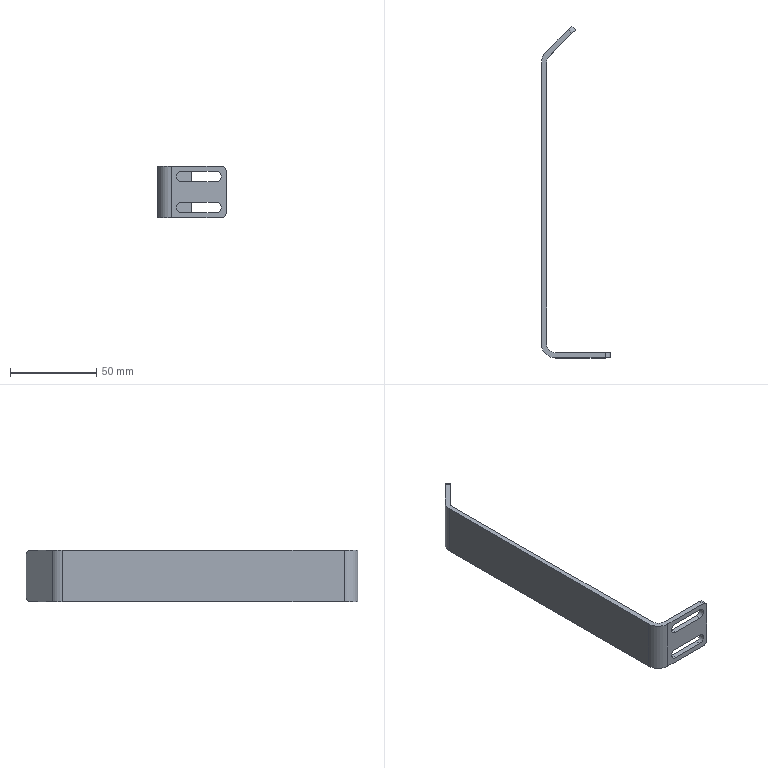Part | NX | features BREP 1 | 1 solid | 26 faces | box 40 x 192.678 x 30 mm | volume 20029 mm3 | plane 14 | cylinder 12 | commonest cylinder face diameters 6 x8 10 x2 16 x2
STEP:
#1=CARTESIAN_POINT('',(0.,8.,30.));
#2=VERTEX_POINT('',#1);
#3=CARTESIAN_POINT('',(0.,171.686,30.));
#4=VERTEX_POINT('',#3);
#5=CARTESIAN_POINT('',(0.,0.,30.));
#6=DIRECTION('',(0.,1.,0.));
#7=VECTOR('',#6,1000.);
#8=LINE('',#5,#7);
#9=EDGE_CURVE('',#2,#4,#8,.T.);
#10=ORIENTED_EDGE('',*,*,#9,.T.);
#11=CARTESIAN_POINT('',(0.,171.686,0.));
#12=VERTEX_POINT('',#11);
#13=CARTESIAN_POINT('',(0.,171.686,30.));
#14=DIRECTION('',(0.,0.,-1.));
#15=VECTOR('',#14,1000.);
#16=LINE('',#13,#15);
#17=EDGE_CURVE('',#4,#12,#16,.T.);
#18=ORIENTED_EDGE('',*,*,#17,.T.);
#19=CARTESIAN_POINT('',(0.,8.,0.));
#20=VERTEX_POINT('',#19);
#21=CARTESIAN_POINT('',(0.,0.,0.));
#22=DIRECTION('',(0.,-1.,0.));
#23=VECTOR('',#22,1000.);
#24=LINE('',#21,#23);
#25=EDGE_CURVE('',#12,#20,#24,.T.);
#26=ORIENTED_EDGE('',*,*,#25,.T.);
#27=CARTESIAN_POINT('',(0.,8.,30.));
#28=DIRECTION('',(0.,0.,1.));
#29=VECTOR('',#28,1000.);
#30=LINE('',#27,#29);
#31=EDGE_CURVE('',#20,#2,#30,.T.);
#32=ORIENTED_EDGE('',*,*,#31,.T.);
#33=EDGE_LOOP('',(#10,#18,#26,#32));
#34=FACE_BOUND('',#33,.T.);
#35=CARTESIAN_POINT('',(0.,0.,30.));
#36=DIRECTION('',(-1.,0.,0.));
#37=DIRECTION('',(0.,0.,-1.));
#38=AXIS2_PLACEMENT_3D('',#35,#36,#37);
#39=PLANE('',#38);
#40=ADVANCED_FACE('',(#34),#39,.T.);
#41=CARTESIAN_POINT('',(2.343,177.343,30.));
#42=VERTEX_POINT('',#41);
#43=CARTESIAN_POINT('',(8.,171.686,30.));
#44=DIRECTION('',(0.,0.,-1.));
#45=DIRECTION('',(-1.,0.,0.));
#46=AXIS2_PLACEMENT_3D('',#43,#44,#45);
#47=CIRCLE('',#46,8.);
#48=EDGE_CURVE('',#4,#42,#47,.T.);
#49=ORIENTED_EDGE('',*,*,#48,.T.);
#50=CARTESIAN_POINT('',(2.343,177.343,0.));
#51=VERTEX_POINT('',#50);
#52=CARTESIAN_POINT('',(2.343,177.343,30.));
#53=DIRECTION('',(0.,0.,-1.));
#54=VECTOR('',#53,1000.);
#55=LINE('',#52,#54);
#56=EDGE_CURVE('',#42,#51,#55,.T.);
#57=ORIENTED_EDGE('',*,*,#56,.T.);
#58=CARTESIAN_POINT('',(8.,171.686,0.));
#59=DIRECTION('',(0.,0.,1.));
#60=DIRECTION('',(-1.,0.,0.));
#61=AXIS2_PLACEMENT_3D('',#58,#59,#60);
#62=CIRCLE('',#61,8.);
#63=EDGE_CURVE('',#51,#12,#62,.T.);
#64=ORIENTED_EDGE('',*,*,#63,.T.);
#65=ORIENTED_EDGE('',*,*,#17,.F.);
#66=EDGE_LOOP('',(#49,#57,#64,#65));
#67=FACE_BOUND('',#66,.T.);
#68=CARTESIAN_POINT('',(8.,171.686,30.));
#69=DIRECTION('',(0.,0.,-1.));
#70=DIRECTION('',(1.,0.,0.));
#71=AXIS2_PLACEMENT_3D('',#68,#69,#70);
#72=CYLINDRICAL_SURFACE('',#71,8.);
#73=ADVANCED_FACE('',(#67),#72,.T.);
#74=CARTESIAN_POINT('',(3.,8.,30.));
#75=VERTEX_POINT('',#74);
#76=CARTESIAN_POINT('',(3.,171.686,30.));
#77=VERTEX_POINT('',#76);
#78=CARTESIAN_POINT('',(3.,3.,30.));
#79=DIRECTION('',(0.,1.,0.));
#80=VECTOR('',#79,1000.);
#81=LINE('',#78,#80);
#82=EDGE_CURVE('',#75,#77,#81,.T.);
#83=ORIENTED_EDGE('',*,*,#82,.T.);
#84=CARTESIAN_POINT('',(4.464,175.222,30.));
#85=VERTEX_POINT('',#84);
#86=CARTESIAN_POINT('',(8.,171.686,30.));
#87=DIRECTION('',(0.,0.,-1.));
#88=DIRECTION('',(-1.,0.,0.));
#89=AXIS2_PLACEMENT_3D('',#86,#87,#88);
#90=CIRCLE('',#89,5.);
#91=EDGE_CURVE('',#77,#85,#90,.T.);
#92=ORIENTED_EDGE('',*,*,#91,.T.);
#93=CARTESIAN_POINT('',(17.678,188.435,30.));
#94=VERTEX_POINT('',#93);
#95=CARTESIAN_POINT('',(4.464,175.222,30.));
#96=DIRECTION('',(0.7071,0.7071,0.));
#97=VECTOR('',#96,1000.);
#98=LINE('',#95,#97);
#99=EDGE_CURVE('',#85,#94,#98,.T.);
#100=ORIENTED_EDGE('',*,*,#99,.T.);
#101=CARTESIAN_POINT('',(15.556,190.556,30.));
#102=VERTEX_POINT('',#101);
#103=CARTESIAN_POINT('',(15.556,190.556,30.));
#104=DIRECTION('',(0.7071,-0.7071,0.));
#105=VECTOR('',#104,1000.);
#106=LINE('',#103,#105);
#107=EDGE_CURVE('',#102,#94,#106,.T.);
#108=ORIENTED_EDGE('',*,*,#107,.F.);
#109=CARTESIAN_POINT('',(0.,175.,30.));
#110=DIRECTION('',(0.7071,0.7071,0.));
#111=VECTOR('',#110,1000.);
#112=LINE('',#109,#111);
#113=EDGE_CURVE('',#42,#102,#112,.T.);
#114=ORIENTED_EDGE('',*,*,#113,.F.);
#115=ORIENTED_EDGE('',*,*,#48,.F.);
#116=ORIENTED_EDGE('',*,*,#9,.F.);
#117=CARTESIAN_POINT('',(8.,0.,30.));
#118=VERTEX_POINT('',#117);
#119=CARTESIAN_POINT('',(8.,8.,30.));
#120=DIRECTION('',(0.,0.,-1.));
#121=DIRECTION('',(-1.,0.,0.));
#122=AXIS2_PLACEMENT_3D('',#119,#120,#121);
#123=CIRCLE('',#122,8.);
#124=EDGE_CURVE('',#118,#2,#123,.T.);
#125=ORIENTED_EDGE('',*,*,#124,.F.);
#126=CARTESIAN_POINT('',(37.,0.,30.));
#127=VERTEX_POINT('',#126);
#128=CARTESIAN_POINT('',(40.,0.,30.));
#129=DIRECTION('',(-1.,0.,0.));
#130=VECTOR('',#129,1000.);
#131=LINE('',#128,#130);
#132=EDGE_CURVE('',#127,#118,#131,.T.);
#133=ORIENTED_EDGE('',*,*,#132,.F.);
#134=CARTESIAN_POINT('',(37.,3.,30.));
#135=VERTEX_POINT('',#134);
#136=CARTESIAN_POINT('',(37.,171.686,30.));
#137=DIRECTION('',(0.,1.,0.));
#138=VECTOR('',#137,1000.);
#139=LINE('',#136,#138);
#140=EDGE_CURVE('',#127,#135,#139,.T.);
#141=ORIENTED_EDGE('',*,*,#140,.T.);
#142=CARTESIAN_POINT('',(8.,3.,30.));
#143=VERTEX_POINT('',#142);
#144=CARTESIAN_POINT('',(8.,3.,30.));
#145=DIRECTION('',(-1.,0.,0.));
#146=VECTOR('',#145,1000.);
#147=LINE('',#144,#146);
#148=EDGE_CURVE('',#135,#143,#147,.T.);
#149=ORIENTED_EDGE('',*,*,#148,.T.);
#150=CARTESIAN_POINT('',(8.,8.,30.));
#151=DIRECTION('',(0.,0.,-1.));
#152=DIRECTION('',(-1.,0.,0.));
#153=AXIS2_PLACEMENT_3D('',#150,#151,#152);
#154=CIRCLE('',#153,5.);
#155=EDGE_CURVE('',#143,#75,#154,.T.);
#156=ORIENTED_EDGE('',*,*,#155,.T.);
#157=EDGE_LOOP('',(#83,#92,#100,#108,#114,#115,#116,#125,#133,#141,#149,#156));
#158=FACE_BOUND('',#157,.T.);
#159=CARTESIAN_POINT('',(8.,3.,30.));
#160=DIRECTION('',(0.,0.,1.));
#161=DIRECTION('',(-1.,0.,0.));
#162=AXIS2_PLACEMENT_3D('',#159,#160,#161);
#163=PLANE('',#162);
#164=ADVANCED_FACE('',(#158),#163,.T.);
#165=ORIENTED_EDGE('',*,*,#124,.T.);
#166=ORIENTED_EDGE('',*,*,#31,.F.);
#167=CARTESIAN_POINT('',(8.,0.,0.));
#168=VERTEX_POINT('',#167);
#169=CARTESIAN_POINT('',(8.,8.,0.));
#170=DIRECTION('',(0.,0.,1.));
#171=DIRECTION('',(-1.,0.,0.));
#172=AXIS2_PLACEMENT_3D('',#169,#170,#171);
#173=CIRCLE('',#172,8.);
#174=EDGE_CURVE('',#20,#168,#173,.T.);
#175=ORIENTED_EDGE('',*,*,#174,.T.);
#176=CARTESIAN_POINT('',(8.,0.,30.));
#177=DIRECTION('',(0.,0.,1.));
#178=VECTOR('',#177,1000.);
#179=LINE('',#176,#178);
#180=EDGE_CURVE('',#168,#118,#179,.T.);
#181=ORIENTED_EDGE('',*,*,#180,.T.);
#182=EDGE_LOOP('',(#165,#166,#175,#181));
#183=FACE_BOUND('',#182,.T.);
#184=CARTESIAN_POINT('',(8.,8.,30.));
#185=DIRECTION('',(0.,0.,-1.));
#186=DIRECTION('',(1.,0.,0.));
#187=AXIS2_PLACEMENT_3D('',#184,#185,#186);
#188=CYLINDRICAL_SURFACE('',#187,8.);
#189=ADVANCED_FACE('',(#183),#188,.T.);
#190=CARTESIAN_POINT('',(3.,171.686,0.));
#191=VERTEX_POINT('',#190);
#192=CARTESIAN_POINT('',(3.,8.,0.));
#193=VERTEX_POINT('',#192);
#194=CARTESIAN_POINT('',(3.,175.222,0.));
#195=DIRECTION('',(0.,-1.,0.));
#196=VECTOR('',#195,1000.);
#197=LINE('',#194,#196);
#198=EDGE_CURVE('',#191,#193,#197,.T.);
#199=ORIENTED_EDGE('',*,*,#198,.T.);
#200=CARTESIAN_POINT('',(8.,3.,0.));
#201=VERTEX_POINT('',#200);
#202=CARTESIAN_POINT('',(8.,8.,0.));
#203=DIRECTION('',(0.,0.,1.));
#204=DIRECTION('',(-1.,0.,0.));
#205=AXIS2_PLACEMENT_3D('',#202,#203,#204);
#206=CIRCLE('',#205,5.);
#207=EDGE_CURVE('',#193,#201,#206,.T.);
#208=ORIENTED_EDGE('',*,*,#207,.T.);
#209=CARTESIAN_POINT('',(37.,3.,0.));
#210=VERTEX_POINT('',#209);
#211=CARTESIAN_POINT('',(3.,3.,0.));
#212=DIRECTION('',(1.,0.,0.));
#213=VECTOR('',#212,1000.);
#214=LINE('',#211,#213);
#215=EDGE_CURVE('',#201,#210,#214,.T.);
#216=ORIENTED_EDGE('',*,*,#215,.T.);
#217=CARTESIAN_POINT('',(37.,0.,0.));
#218=VERTEX_POINT('',#217);
#219=CARTESIAN_POINT('',(37.,8.,0.));
#220=DIRECTION('',(0.,1.,0.));
#221=VECTOR('',#220,1000.);
#222=LINE('',#219,#221);
#223=EDGE_CURVE('',#218,#210,#222,.T.);
#224=ORIENTED_EDGE('',*,*,#223,.F.);
#225=CARTESIAN_POINT('',(40.,0.,0.));
#226=DIRECTION('',(1.,0.,0.));
#227=VECTOR('',#226,1000.);
#228=LINE('',#225,#227);
#229=EDGE_CURVE('',#168,#218,#228,.T.);
#230=ORIENTED_EDGE('',*,*,#229,.F.);
#231=ORIENTED_EDGE('',*,*,#174,.F.);
#232=ORIENTED_EDGE('',*,*,#25,.F.);
#233=ORIENTED_EDGE('',*,*,#63,.F.);
#234=CARTESIAN_POINT('',(15.556,190.556,0.));
#235=VERTEX_POINT('',#234);
#236=CARTESIAN_POINT('',(0.,175.,0.));
#237=DIRECTION('',(-0.7071,-0.7071,0.));
#238=VECTOR('',#237,1000.);
#239=LINE('',#236,#238);
#240=EDGE_CURVE('',#235,#51,#239,.T.);
#241=ORIENTED_EDGE('',*,*,#240,.F.);
#242=CARTESIAN_POINT('',(17.678,188.435,0.));
#243=VERTEX_POINT('',#242);
#244=CARTESIAN_POINT('',(17.678,188.435,0.));
#245=DIRECTION('',(-0.7071,0.7071,0.));
#246=VECTOR('',#245,1000.);
#247=LINE('',#244,#246);
#248=EDGE_CURVE('',#243,#235,#247,.T.);
#249=ORIENTED_EDGE('',*,*,#248,.F.);
#250=CARTESIAN_POINT('',(4.464,175.222,0.));
#251=VERTEX_POINT('',#250);
#252=CARTESIAN_POINT('',(4.464,175.222,0.));
#253=DIRECTION('',(0.7071,0.7071,0.));
#254=VECTOR('',#253,1000.);
#255=LINE('',#252,#254);
#256=EDGE_CURVE('',#251,#243,#255,.T.);
#257=ORIENTED_EDGE('',*,*,#256,.F.);
#258=CARTESIAN_POINT('',(8.,171.686,0.));
#259=DIRECTION('',(0.,0.,1.));
#260=DIRECTION('',(-1.,0.,0.));
#261=AXIS2_PLACEMENT_3D('',#258,#259,#260);
#262=CIRCLE('',#261,5.);
#263=EDGE_CURVE('',#251,#191,#262,.T.);
#264=ORIENTED_EDGE('',*,*,#263,.T.);
#265=EDGE_LOOP('',(#199,#208,#216,#224,#230,#231,#232,#233,#241,#249,#257,#264));
#266=FACE_BOUND('',#265,.T.);
#267=CARTESIAN_POINT('',(4.464,175.222,0.));
#268=DIRECTION('',(0.,0.,-1.));
#269=DIRECTION('',(1.,0.,0.));
#270=AXIS2_PLACEMENT_3D('',#267,#268,#269);
#271=PLANE('',#270);
#272=ADVANCED_FACE('',(#266),#271,.T.);
#273=ORIENTED_EDGE('',*,*,#240,.T.);
#274=ORIENTED_EDGE('',*,*,#56,.F.);
#275=ORIENTED_EDGE('',*,*,#113,.T.);
#276=CARTESIAN_POINT('',(17.678,192.678,27.));
#277=VERTEX_POINT('',#276);
#278=CARTESIAN_POINT('',(15.556,190.556,27.));
#279=DIRECTION('',(-0.7071,0.7071,0.));
#280=DIRECTION('',(0.7071,0.7071,0.));
#281=AXIS2_PLACEMENT_3D('',#278,#279,#280);
#282=CIRCLE('',#281,3.);
#283=EDGE_CURVE('',#102,#277,#282,.T.);
#284=ORIENTED_EDGE('',*,*,#283,.T.);
#285=CARTESIAN_POINT('',(17.678,192.678,3.));
#286=VERTEX_POINT('',#285);
#287=CARTESIAN_POINT('',(17.678,192.678,30.));
#288=DIRECTION('',(0.,0.,-1.));
#289=VECTOR('',#288,1000.);
#290=LINE('',#287,#289);
#291=EDGE_CURVE('',#277,#286,#290,.T.);
#292=ORIENTED_EDGE('',*,*,#291,.T.);
#293=CARTESIAN_POINT('',(15.556,190.556,3.));
#294=DIRECTION('',(-0.7071,0.7071,0.));
#295=DIRECTION('',(-0.7071,-0.7071,0.));
#296=AXIS2_PLACEMENT_3D('',#293,#294,#295);
#297=CIRCLE('',#296,3.);
#298=EDGE_CURVE('',#286,#235,#297,.T.);
#299=ORIENTED_EDGE('',*,*,#298,.T.);
#300=EDGE_LOOP('',(#273,#274,#275,#284,#292,#299));
#301=FACE_BOUND('',#300,.T.);
#302=CARTESIAN_POINT('',(0.,175.,30.));
#303=DIRECTION('',(-0.7071,0.7071,0.));
#304=DIRECTION('',(0.7071,0.7071,0.));
#305=AXIS2_PLACEMENT_3D('',#302,#303,#304);
#306=PLANE('',#305);
#307=ADVANCED_FACE('',(#301),#306,.T.);
#308=CARTESIAN_POINT('',(3.,171.686,30.));
#309=DIRECTION('',(0.,0.,-1.));
#310=VECTOR('',#309,1000.);
#311=LINE('',#308,#310);
#312=EDGE_CURVE('',#77,#191,#311,.T.);
#313=ORIENTED_EDGE('',*,*,#312,.F.);
#314=ORIENTED_EDGE('',*,*,#82,.F.);
#315=CARTESIAN_POINT('',(3.,8.,30.));
#316=DIRECTION('',(0.,0.,1.));
#317=VECTOR('',#316,1000.);
#318=LINE('',#315,#317);
#319=EDGE_CURVE('',#193,#75,#318,.T.);
#320=ORIENTED_EDGE('',*,*,#319,.F.);
#321=ORIENTED_EDGE('',*,*,#198,.F.);
#322=EDGE_LOOP('',(#313,#314,#320,#321));
#323=FACE_BOUND('',#322,.T.);
#324=CARTESIAN_POINT('',(3.,0.,30.));
#325=DIRECTION('',(-1.,0.,0.));
#326=DIRECTION('',(0.,0.,-1.));
#327=AXIS2_PLACEMENT_3D('',#324,#325,#326);
#328=PLANE('',#327);
#329=ADVANCED_FACE('',(#323),#328,.F.);
#330=ORIENTED_EDGE('',*,*,#229,.T.);
#331=CARTESIAN_POINT('',(40.,0.,3.));
#332=VERTEX_POINT('',#331);
#333=CARTESIAN_POINT('',(37.,0.,3.));
#334=DIRECTION('',(0.,-1.,0.));
#335=DIRECTION('',(0.,0.,-1.));
#336=AXIS2_PLACEMENT_3D('',#333,#334,#335);
#337=CIRCLE('',#336,3.);
#338=EDGE_CURVE('',#218,#332,#337,.T.);
#339=ORIENTED_EDGE('',*,*,#338,.T.);
#340=CARTESIAN_POINT('',(40.,0.,27.));
#341=VERTEX_POINT('',#340);
#342=CARTESIAN_POINT('',(40.,0.,30.));
#343=DIRECTION('',(0.,0.,1.));
#344=VECTOR('',#343,1000.);
#345=LINE('',#342,#344);
#346=EDGE_CURVE('',#332,#341,#345,.T.);
#347=ORIENTED_EDGE('',*,*,#346,.T.);
#348=CARTESIAN_POINT('',(37.,0.,27.));
#349=DIRECTION('',(0.,-1.,0.));
#350=DIRECTION('',(0.,0.,-1.));
#351=AXIS2_PLACEMENT_3D('',#348,#349,#350);
#352=CIRCLE('',#351,3.);
#353=EDGE_CURVE('',#341,#127,#352,.T.);
#354=ORIENTED_EDGE('',*,*,#353,.T.);
#355=ORIENTED_EDGE('',*,*,#132,.T.);
#356=ORIENTED_EDGE('',*,*,#180,.F.);
#357=EDGE_LOOP('',(#330,#339,#347,#354,#355,#356));
#358=FACE_BOUND('',#357,.T.);
#359=CARTESIAN_POINT('',(34.,0.,9.));
#360=VERTEX_POINT('',#359);
#361=CARTESIAN_POINT('',(34.,0.,3.));
#362=VERTEX_POINT('',#361);
#363=CARTESIAN_POINT('',(34.,0.,6.));
#364=DIRECTION('',(0.,1.,0.));
#365=DIRECTION('',(1.,0.,0.));
#366=AXIS2_PLACEMENT_3D('',#363,#364,#365);
#367=CIRCLE('',#366,3.);
#368=EDGE_CURVE('',#360,#362,#367,.T.);
#369=ORIENTED_EDGE('',*,*,#368,.T.);
#370=CARTESIAN_POINT('',(14.,0.,3.));
#371=VERTEX_POINT('',#370);
#372=CARTESIAN_POINT('',(40.,0.,3.));
#373=DIRECTION('',(-1.,0.,0.));
#374=VECTOR('',#373,1000.);
#375=LINE('',#372,#374);
#376=EDGE_CURVE('',#362,#371,#375,.T.);
#377=ORIENTED_EDGE('',*,*,#376,.T.);
#378=CARTESIAN_POINT('',(14.,0.,9.));
#379=VERTEX_POINT('',#378);
#380=CARTESIAN_POINT('',(14.,0.,6.));
#381=DIRECTION('',(0.,1.,0.));
#382=DIRECTION('',(1.,0.,0.));
#383=AXIS2_PLACEMENT_3D('',#380,#381,#382);
#384=CIRCLE('',#383,3.);
#385=EDGE_CURVE('',#371,#379,#384,.T.);
#386=ORIENTED_EDGE('',*,*,#385,.T.);
#387=CARTESIAN_POINT('',(40.,0.,9.));
#388=DIRECTION('',(1.,0.,0.));
#389=VECTOR('',#388,1000.);
#390=LINE('',#387,#389);
#391=EDGE_CURVE('',#379,#360,#390,.T.);
#392=ORIENTED_EDGE('',*,*,#391,.T.);
#393=EDGE_LOOP('',(#369,#377,#386,#392));
#394=FACE_BOUND('',#393,.T.);
#395=CARTESIAN_POINT('',(34.,0.,27.));
#396=VERTEX_POINT('',#395);
#397=CARTESIAN_POINT('',(34.,0.,21.));
#398=VERTEX_POINT('',#397);
#399=CARTESIAN_POINT('',(34.,0.,24.));
#400=DIRECTION('',(0.,1.,0.));
#401=DIRECTION('',(1.,0.,0.));
#402=AXIS2_PLACEMENT_3D('',#399,#400,#401);
#403=CIRCLE('',#402,3.);
#404=EDGE_CURVE('',#396,#398,#403,.T.);
#405=ORIENTED_EDGE('',*,*,#404,.T.);
#406=CARTESIAN_POINT('',(14.,0.,21.));
#407=VERTEX_POINT('',#406);
#408=CARTESIAN_POINT('',(40.,0.,21.));
#409=DIRECTION('',(-1.,0.,0.));
#410=VECTOR('',#409,1000.);
#411=LINE('',#408,#410);
#412=EDGE_CURVE('',#398,#407,#411,.T.);
#413=ORIENTED_EDGE('',*,*,#412,.T.);
#414=CARTESIAN_POINT('',(14.,0.,27.));
#415=VERTEX_POINT('',#414);
#416=CARTESIAN_POINT('',(14.,0.,24.));
#417=DIRECTION('',(0.,1.,0.));
#418=DIRECTION('',(1.,0.,0.));
#419=AXIS2_PLACEMENT_3D('',#416,#417,#418);
#420=CIRCLE('',#419,3.);
#421=EDGE_CURVE('',#407,#415,#420,.T.);
#422=ORIENTED_EDGE('',*,*,#421,.T.);
#423=CARTESIAN_POINT('',(40.,0.,27.));
#424=DIRECTION('',(1.,0.,0.));
#425=VECTOR('',#424,1000.);
#426=LINE('',#423,#425);
#427=EDGE_CURVE('',#415,#396,#426,.T.);
#428=ORIENTED_EDGE('',*,*,#427,.T.);
#429=EDGE_LOOP('',(#405,#413,#422,#428));
#430=FACE_BOUND('',#429,.T.);
#431=CARTESIAN_POINT('',(40.,0.,30.));
#432=DIRECTION('',(0.,-1.,0.));
#433=DIRECTION('',(-1.,0.,0.));
#434=AXIS2_PLACEMENT_3D('',#431,#432,#433);
#435=PLANE('',#434);
#436=ADVANCED_FACE('',(#358,#394,#430),#435,.T.);
#437=CARTESIAN_POINT('',(19.799,190.556,3.));
#438=VERTEX_POINT('',#437);
#439=CARTESIAN_POINT('',(17.678,188.435,3.));
#440=DIRECTION('',(-0.7071,0.7071,0.));
#441=DIRECTION('',(-0.7071,-0.7071,0.));
#442=AXIS2_PLACEMENT_3D('',#439,#440,#441);
#443=CIRCLE('',#442,3.);
#444=EDGE_CURVE('',#438,#243,#443,.T.);
#445=ORIENTED_EDGE('',*,*,#444,.T.);
#446=ORIENTED_EDGE('',*,*,#248,.T.);
#447=ORIENTED_EDGE('',*,*,#298,.F.);
#448=CARTESIAN_POINT('',(23.335,187.021,3.));
#449=DIRECTION('',(0.7071,-0.7071,0.));
#450=VECTOR('',#449,1000.);
#451=LINE('',#448,#450);
#452=EDGE_CURVE('',#286,#438,#451,.T.);
#453=ORIENTED_EDGE('',*,*,#452,.T.);
#454=EDGE_LOOP('',(#445,#446,#447,#453));
#455=FACE_BOUND('',#454,.T.);
#456=CARTESIAN_POINT('',(21.213,184.899,3.));
#457=DIRECTION('',(-0.7071,0.7071,0.));
#458=DIRECTION('',(0.7071,0.7071,0.));
#459=AXIS2_PLACEMENT_3D('',#456,#457,#458);
#460=CYLINDRICAL_SURFACE('',#459,3.);
#461=ADVANCED_FACE('',(#455),#460,.T.);
#462=CARTESIAN_POINT('',(19.799,190.556,27.));
#463=VERTEX_POINT('',#462);
#464=CARTESIAN_POINT('',(19.799,190.556,30.));
#465=DIRECTION('',(0.,0.,-1.));
#466=VECTOR('',#465,1000.);
#467=LINE('',#464,#466);
#468=EDGE_CURVE('',#463,#438,#467,.T.);
#469=ORIENTED_EDGE('',*,*,#468,.T.);
#470=ORIENTED_EDGE('',*,*,#452,.F.);
#471=ORIENTED_EDGE('',*,*,#291,.F.);
#472=CARTESIAN_POINT('',(17.678,192.678,27.));
#473=DIRECTION('',(0.7071,-0.7071,0.));
#474=VECTOR('',#473,1000.);
#475=LINE('',#472,#474);
#476=EDGE_CURVE('',#277,#463,#475,.T.);
#477=ORIENTED_EDGE('',*,*,#476,.T.);
#478=EDGE_LOOP('',(#469,#470,#471,#477));
#479=FACE_BOUND('',#478,.T.);
#480=CARTESIAN_POINT('',(17.678,192.678,30.));
#481=DIRECTION('',(0.7071,0.7071,0.));
#482=DIRECTION('',(0.7071,-0.7071,0.));
#483=AXIS2_PLACEMENT_3D('',#480,#481,#482);
#484=PLANE('',#483);
#485=ADVANCED_FACE('',(#479),#484,.T.);
#486=CARTESIAN_POINT('',(17.678,188.435,27.));
#487=DIRECTION('',(-0.7071,0.7071,0.));
#488=DIRECTION('',(0.7071,0.7071,0.));
#489=AXIS2_PLACEMENT_3D('',#486,#487,#488);
#490=CIRCLE('',#489,3.);
#491=EDGE_CURVE('',#94,#463,#490,.T.);
#492=ORIENTED_EDGE('',*,*,#491,.T.);
#493=ORIENTED_EDGE('',*,*,#476,.F.);
#494=ORIENTED_EDGE('',*,*,#283,.F.);
#495=ORIENTED_EDGE('',*,*,#107,.T.);
#496=EDGE_LOOP('',(#492,#493,#494,#495));
#497=FACE_BOUND('',#496,.T.);
#498=CARTESIAN_POINT('',(15.556,190.556,27.));
#499=DIRECTION('',(0.7071,-0.7071,0.));
#500=DIRECTION('',(-0.7071,-0.7071,0.));
#501=AXIS2_PLACEMENT_3D('',#498,#499,#500);
#502=CYLINDRICAL_SURFACE('',#501,3.);
#503=ADVANCED_FACE('',(#497),#502,.T.);
#504=CARTESIAN_POINT('',(4.464,175.222,30.));
#505=DIRECTION('',(0.,0.,-1.));
#506=VECTOR('',#505,1000.);
#507=LINE('',#504,#506);
#508=EDGE_CURVE('',#85,#251,#507,.T.);
#509=ORIENTED_EDGE('',*,*,#508,.F.);
#510=ORIENTED_EDGE('',*,*,#91,.F.);
#511=ORIENTED_EDGE('',*,*,#312,.T.);
#512=ORIENTED_EDGE('',*,*,#263,.F.);
#513=EDGE_LOOP('',(#509,#510,#511,#512));
#514=FACE_BOUND('',#513,.T.);
#515=CARTESIAN_POINT('',(8.,171.686,30.));
#516=DIRECTION('',(0.,0.,-1.));
#517=DIRECTION('',(1.,0.,0.));
#518=AXIS2_PLACEMENT_3D('',#515,#516,#517);
#519=CYLINDRICAL_SURFACE('',#518,5.);
#520=ADVANCED_FACE('',(#514),#519,.F.);
#521=ORIENTED_EDGE('',*,*,#319,.T.);
#522=ORIENTED_EDGE('',*,*,#155,.F.);
#523=CARTESIAN_POINT('',(8.,3.,30.));
#524=DIRECTION('',(0.,0.,1.));
#525=VECTOR('',#524,1000.);
#526=LINE('',#523,#525);
#527=EDGE_CURVE('',#201,#143,#526,.T.);
#528=ORIENTED_EDGE('',*,*,#527,.F.);
#529=ORIENTED_EDGE('',*,*,#207,.F.);
#530=EDGE_LOOP('',(#521,#522,#528,#529));
#531=FACE_BOUND('',#530,.T.);
#532=CARTESIAN_POINT('',(8.,8.,30.));
#533=DIRECTION('',(0.,0.,-1.));
#534=DIRECTION('',(1.,0.,0.));
#535=AXIS2_PLACEMENT_3D('',#532,#533,#534);
#536=CYLINDRICAL_SURFACE('',#535,5.);
#537=ADVANCED_FACE('',(#531),#536,.F.);
#538=ORIENTED_EDGE('',*,*,#338,.F.);
#539=ORIENTED_EDGE('',*,*,#223,.T.);
#540=CARTESIAN_POINT('',(40.,3.,3.));
#541=VERTEX_POINT('',#540);
#542=CARTESIAN_POINT('',(37.,3.,3.));
#543=DIRECTION('',(0.,-1.,0.));
#544=DIRECTION('',(0.,0.,-1.));
#545=AXIS2_PLACEMENT_3D('',#542,#543,#544);
#546=CIRCLE('',#545,3.);
#547=EDGE_CURVE('',#210,#541,#546,.T.);
#548=ORIENTED_EDGE('',*,*,#547,.T.);
#549=CARTESIAN_POINT('',(40.,8.,3.));
#550=DIRECTION('',(0.,-1.,0.));
#551=VECTOR('',#550,1000.);
#552=LINE('',#549,#551);
#553=EDGE_CURVE('',#541,#332,#552,.T.);
#554=ORIENTED_EDGE('',*,*,#553,.T.);
#555=EDGE_LOOP('',(#538,#539,#548,#554));
#556=FACE_BOUND('',#555,.T.);
#557=CARTESIAN_POINT('',(37.,8.,3.));
#558=DIRECTION('',(0.,-1.,0.));
#559=DIRECTION('',(0.,0.,1.));
#560=AXIS2_PLACEMENT_3D('',#557,#558,#559);
#561=CYLINDRICAL_SURFACE('',#560,3.);
#562=ADVANCED_FACE('',(#556),#561,.T.);
#563=ORIENTED_EDGE('',*,*,#353,.F.);
#564=CARTESIAN_POINT('',(40.,3.,27.));
#565=VERTEX_POINT('',#564);
#566=CARTESIAN_POINT('',(40.,3.,27.));
#567=DIRECTION('',(0.,1.,0.));
#568=VECTOR('',#567,1000.);
#569=LINE('',#566,#568);
#570=EDGE_CURVE('',#341,#565,#569,.T.);
#571=ORIENTED_EDGE('',*,*,#570,.T.);
#572=CARTESIAN_POINT('',(37.,3.,27.));
#573=DIRECTION('',(0.,-1.,0.));
#574=DIRECTION('',(0.,0.,-1.));
#575=AXIS2_PLACEMENT_3D('',#572,#573,#574);
#576=CIRCLE('',#575,3.);
#577=EDGE_CURVE('',#565,#135,#576,.T.);
#578=ORIENTED_EDGE('',*,*,#577,.T.);
#579=ORIENTED_EDGE('',*,*,#140,.F.);
#580=EDGE_LOOP('',(#563,#571,#578,#579));
#581=FACE_BOUND('',#580,.T.);
#582=CARTESIAN_POINT('',(37.,3.,27.));
#583=DIRECTION('',(0.,-1.,0.));
#584=DIRECTION('',(0.,0.,1.));
#585=AXIS2_PLACEMENT_3D('',#582,#583,#584);
#586=CYLINDRICAL_SURFACE('',#585,3.);
#587=ADVANCED_FACE('',(#581),#586,.T.);
#588=ORIENTED_EDGE('',*,*,#346,.F.);
#589=ORIENTED_EDGE('',*,*,#553,.F.);
#590=CARTESIAN_POINT('',(40.,3.,30.));
#591=DIRECTION('',(0.,0.,1.));
#592=VECTOR('',#591,1000.);
#593=LINE('',#590,#592);
#594=EDGE_CURVE('',#541,#565,#593,.T.);
#595=ORIENTED_EDGE('',*,*,#594,.T.);
#596=ORIENTED_EDGE('',*,*,#570,.F.);
#597=EDGE_LOOP('',(#588,#589,#595,#596));
#598=FACE_BOUND('',#597,.T.);
#599=CARTESIAN_POINT('',(40.,3.,30.));
#600=DIRECTION('',(1.,0.,0.));
#601=DIRECTION('',(0.,0.,1.));
#602=AXIS2_PLACEMENT_3D('',#599,#600,#601);
#603=PLANE('',#602);
#604=ADVANCED_FACE('',(#598),#603,.T.);
#605=ORIENTED_EDGE('',*,*,#376,.F.);
#606=CARTESIAN_POINT('',(34.,3.,3.));
#607=VERTEX_POINT('',#606);
#608=CARTESIAN_POINT('',(34.,10.,3.));
#609=DIRECTION('',(0.,-1.,0.));
#610=VECTOR('',#609,1000.);
#611=LINE('',#608,#610);
#612=EDGE_CURVE('',#607,#362,#611,.T.);
#613=ORIENTED_EDGE('',*,*,#612,.F.);
#614=CARTESIAN_POINT('',(14.,3.,3.));
#615=VERTEX_POINT('',#614);
#616=CARTESIAN_POINT('',(14.,3.,3.));
#617=DIRECTION('',(1.,0.,0.));
#618=VECTOR('',#617,1000.);
#619=LINE('',#616,#618);
#620=EDGE_CURVE('',#615,#607,#619,.T.);
#621=ORIENTED_EDGE('',*,*,#620,.F.);
#622=CARTESIAN_POINT('',(14.,10.,3.));
#623=DIRECTION('',(0.,1.,0.));
#624=VECTOR('',#623,1000.);
#625=LINE('',#622,#624);
#626=EDGE_CURVE('',#371,#615,#625,.T.);
#627=ORIENTED_EDGE('',*,*,#626,.F.);
#628=EDGE_LOOP('',(#605,#613,#621,#627));
#629=FACE_BOUND('',#628,.T.);
#630=CARTESIAN_POINT('',(14.,10.,3.));
#631=DIRECTION('',(0.,0.,-1.));
#632=DIRECTION('',(1.,0.,0.));
#633=AXIS2_PLACEMENT_3D('',#630,#631,#632);
#634=PLANE('',#633);
#635=ADVANCED_FACE('',(#629),#634,.F.);
#636=CARTESIAN_POINT('',(34.,3.,9.));
#637=VERTEX_POINT('',#636);
#638=CARTESIAN_POINT('',(34.,3.,6.));
#639=DIRECTION('',(0.,-1.,0.));
#640=DIRECTION('',(1.,0.,0.));
#641=AXIS2_PLACEMENT_3D('',#638,#639,#640);
#642=CIRCLE('',#641,3.);
#643=EDGE_CURVE('',#607,#637,#642,.T.);
#644=ORIENTED_EDGE('',*,*,#643,.F.);
#645=ORIENTED_EDGE('',*,*,#612,.T.);
#646=ORIENTED_EDGE('',*,*,#368,.F.);
#647=CARTESIAN_POINT('',(34.,10.,9.));
#648=DIRECTION('',(0.,-1.,0.));
#649=VECTOR('',#648,1000.);
#650=LINE('',#647,#649);
#651=EDGE_CURVE('',#637,#360,#650,.T.);
#652=ORIENTED_EDGE('',*,*,#651,.F.);
#653=EDGE_LOOP('',(#644,#645,#646,#652));
#654=FACE_BOUND('',#653,.T.);
#655=CARTESIAN_POINT('',(34.,10.,6.));
#656=DIRECTION('',(0.,-1.,0.));
#657=DIRECTION('',(-1.,0.,0.));
#658=AXIS2_PLACEMENT_3D('',#655,#656,#657);
#659=CYLINDRICAL_SURFACE('',#658,3.);
#660=ADVANCED_FACE('',(#654),#659,.F.);
#661=ORIENTED_EDGE('',*,*,#391,.F.);
#662=CARTESIAN_POINT('',(14.,3.,9.));
#663=VERTEX_POINT('',#662);
#664=CARTESIAN_POINT('',(14.,10.,9.));
#665=DIRECTION('',(0.,-1.,0.));
#666=VECTOR('',#665,1000.);
#667=LINE('',#664,#666);
#668=EDGE_CURVE('',#663,#379,#667,.T.);
#669=ORIENTED_EDGE('',*,*,#668,.F.);
#670=CARTESIAN_POINT('',(14.,3.,9.));
#671=DIRECTION('',(-1.,0.,0.));
#672=VECTOR('',#671,1000.);
#673=LINE('',#670,#672);
#674=EDGE_CURVE('',#637,#663,#673,.T.);
#675=ORIENTED_EDGE('',*,*,#674,.F.);
#676=ORIENTED_EDGE('',*,*,#651,.T.);
#677=EDGE_LOOP('',(#661,#669,#675,#676));
#678=FACE_BOUND('',#677,.T.);
#679=CARTESIAN_POINT('',(14.,10.,9.));
#680=DIRECTION('',(0.,0.,1.));
#681=DIRECTION('',(-1.,0.,0.));
#682=AXIS2_PLACEMENT_3D('',#679,#680,#681);
#683=PLANE('',#682);
#684=ADVANCED_FACE('',(#678),#683,.F.);
#685=ORIENTED_EDGE('',*,*,#385,.F.);
#686=ORIENTED_EDGE('',*,*,#626,.T.);
#687=CARTESIAN_POINT('',(14.,3.,6.));
#688=DIRECTION('',(0.,-1.,0.));
#689=DIRECTION('',(1.,0.,0.));
#690=AXIS2_PLACEMENT_3D('',#687,#688,#689);
#691=CIRCLE('',#690,3.);
#692=EDGE_CURVE('',#663,#615,#691,.T.);
#693=ORIENTED_EDGE('',*,*,#692,.F.);
#694=ORIENTED_EDGE('',*,*,#668,.T.);
#695=EDGE_LOOP('',(#685,#686,#693,#694));
#696=FACE_BOUND('',#695,.T.);
#697=CARTESIAN_POINT('',(14.,10.,6.));
#698=DIRECTION('',(0.,-1.,0.));
#699=DIRECTION('',(-1.,0.,0.));
#700=AXIS2_PLACEMENT_3D('',#697,#698,#699);
#701=CYLINDRICAL_SURFACE('',#700,3.);
#702=ADVANCED_FACE('',(#696),#701,.F.);
#703=ORIENTED_EDGE('',*,*,#412,.F.);
#704=CARTESIAN_POINT('',(34.,3.,21.));
#705=VERTEX_POINT('',#704);
#706=CARTESIAN_POINT('',(34.,10.,21.));
#707=DIRECTION('',(0.,-1.,0.));
#708=VECTOR('',#707,1000.);
#709=LINE('',#706,#708);
#710=EDGE_CURVE('',#705,#398,#709,.T.);
#711=ORIENTED_EDGE('',*,*,#710,.F.);
#712=CARTESIAN_POINT('',(14.,3.,21.));
#713=VERTEX_POINT('',#712);
#714=CARTESIAN_POINT('',(14.,3.,21.));
#715=DIRECTION('',(1.,0.,0.));
#716=VECTOR('',#715,1000.);
#717=LINE('',#714,#716);
#718=EDGE_CURVE('',#713,#705,#717,.T.);
#719=ORIENTED_EDGE('',*,*,#718,.F.);
#720=CARTESIAN_POINT('',(14.,10.,21.));
#721=DIRECTION('',(0.,1.,0.));
#722=VECTOR('',#721,1000.);
#723=LINE('',#720,#722);
#724=EDGE_CURVE('',#407,#713,#723,.T.);
#725=ORIENTED_EDGE('',*,*,#724,.F.);
#726=EDGE_LOOP('',(#703,#711,#719,#725));
#727=FACE_BOUND('',#726,.T.);
#728=CARTESIAN_POINT('',(14.,10.,21.));
#729=DIRECTION('',(0.,0.,-1.));
#730=DIRECTION('',(1.,0.,0.));
#731=AXIS2_PLACEMENT_3D('',#728,#729,#730);
#732=PLANE('',#731);
#733=ADVANCED_FACE('',(#727),#732,.F.);
#734=CARTESIAN_POINT('',(34.,3.,27.));
#735=VERTEX_POINT('',#734);
#736=CARTESIAN_POINT('',(34.,3.,24.));
#737=DIRECTION('',(0.,-1.,0.));
#738=DIRECTION('',(1.,0.,0.));
#739=AXIS2_PLACEMENT_3D('',#736,#737,#738);
#740=CIRCLE('',#739,3.);
#741=EDGE_CURVE('',#705,#735,#740,.T.);
#742=ORIENTED_EDGE('',*,*,#741,.F.);
#743=ORIENTED_EDGE('',*,*,#710,.T.);
#744=ORIENTED_EDGE('',*,*,#404,.F.);
#745=CARTESIAN_POINT('',(34.,10.,27.));
#746=DIRECTION('',(0.,-1.,0.));
#747=VECTOR('',#746,1000.);
#748=LINE('',#745,#747);
#749=EDGE_CURVE('',#735,#396,#748,.T.);
#750=ORIENTED_EDGE('',*,*,#749,.F.);
#751=EDGE_LOOP('',(#742,#743,#744,#750));
#752=FACE_BOUND('',#751,.T.);
#753=CARTESIAN_POINT('',(34.,10.,24.));
#754=DIRECTION('',(0.,-1.,0.));
#755=DIRECTION('',(-1.,0.,0.));
#756=AXIS2_PLACEMENT_3D('',#753,#754,#755);
#757=CYLINDRICAL_SURFACE('',#756,3.);
#758=ADVANCED_FACE('',(#752),#757,.F.);
#759=ORIENTED_EDGE('',*,*,#427,.F.);
#760=CARTESIAN_POINT('',(14.,3.,27.));
#761=VERTEX_POINT('',#760);
#762=CARTESIAN_POINT('',(14.,10.,27.));
#763=DIRECTION('',(0.,-1.,0.));
#764=VECTOR('',#763,1000.);
#765=LINE('',#762,#764);
#766=EDGE_CURVE('',#761,#415,#765,.T.);
#767=ORIENTED_EDGE('',*,*,#766,.F.);
#768=CARTESIAN_POINT('',(14.,3.,27.));
#769=DIRECTION('',(-1.,0.,0.));
#770=VECTOR('',#769,1000.);
#771=LINE('',#768,#770);
#772=EDGE_CURVE('',#735,#761,#771,.T.);
#773=ORIENTED_EDGE('',*,*,#772,.F.);
#774=ORIENTED_EDGE('',*,*,#749,.T.);
#775=EDGE_LOOP('',(#759,#767,#773,#774));
#776=FACE_BOUND('',#775,.T.);
#777=CARTESIAN_POINT('',(14.,10.,27.));
#778=DIRECTION('',(0.,0.,1.));
#779=DIRECTION('',(-1.,0.,0.));
#780=AXIS2_PLACEMENT_3D('',#777,#778,#779);
#781=PLANE('',#780);
#782=ADVANCED_FACE('',(#776),#781,.F.);
#783=ORIENTED_EDGE('',*,*,#421,.F.);
#784=ORIENTED_EDGE('',*,*,#724,.T.);
#785=CARTESIAN_POINT('',(14.,3.,24.));
#786=DIRECTION('',(0.,-1.,0.));
#787=DIRECTION('',(1.,0.,0.));
#788=AXIS2_PLACEMENT_3D('',#785,#786,#787);
#789=CIRCLE('',#788,3.);
#790=EDGE_CURVE('',#761,#713,#789,.T.);
#791=ORIENTED_EDGE('',*,*,#790,.F.);
#792=ORIENTED_EDGE('',*,*,#766,.T.);
#793=EDGE_LOOP('',(#783,#784,#791,#792));
#794=FACE_BOUND('',#793,.T.);
#795=CARTESIAN_POINT('',(14.,10.,24.));
#796=DIRECTION('',(0.,-1.,0.));
#797=DIRECTION('',(-1.,0.,0.));
#798=AXIS2_PLACEMENT_3D('',#795,#796,#797);
#799=CYLINDRICAL_SURFACE('',#798,3.);
#800=ADVANCED_FACE('',(#794),#799,.F.);
#801=ORIENTED_EDGE('',*,*,#491,.F.);
#802=ORIENTED_EDGE('',*,*,#99,.F.);
#803=ORIENTED_EDGE('',*,*,#508,.T.);
#804=ORIENTED_EDGE('',*,*,#256,.T.);
#805=ORIENTED_EDGE('',*,*,#444,.F.);
#806=ORIENTED_EDGE('',*,*,#468,.F.);
#807=EDGE_LOOP('',(#801,#802,#803,#804,#805,#806));
#808=FACE_BOUND('',#807,.T.);
#809=CARTESIAN_POINT('',(2.121,172.879,30.));
#810=DIRECTION('',(-0.7071,0.7071,0.));
#811=DIRECTION('',(0.7071,0.7071,0.));
#812=AXIS2_PLACEMENT_3D('',#809,#810,#811);
#813=PLANE('',#812);
#814=ADVANCED_FACE('',(#808),#813,.F.);
#815=ORIENTED_EDGE('',*,*,#577,.F.);
#816=ORIENTED_EDGE('',*,*,#594,.F.);
#817=ORIENTED_EDGE('',*,*,#547,.F.);
#818=ORIENTED_EDGE('',*,*,#215,.F.);
#819=ORIENTED_EDGE('',*,*,#527,.T.);
#820=ORIENTED_EDGE('',*,*,#148,.F.);
#821=EDGE_LOOP('',(#815,#816,#817,#818,#819,#820));
#822=FACE_BOUND('',#821,.T.);
#823=ORIENTED_EDGE('',*,*,#692,.T.);
#824=ORIENTED_EDGE('',*,*,#620,.T.);
#825=ORIENTED_EDGE('',*,*,#643,.T.);
#826=ORIENTED_EDGE('',*,*,#674,.T.);
#827=EDGE_LOOP('',(#823,#824,#825,#826));
#828=FACE_BOUND('',#827,.T.);
#829=ORIENTED_EDGE('',*,*,#790,.T.);
#830=ORIENTED_EDGE('',*,*,#718,.T.);
#831=ORIENTED_EDGE('',*,*,#741,.T.);
#832=ORIENTED_EDGE('',*,*,#772,.T.);
#833=EDGE_LOOP('',(#829,#830,#831,#832));
#834=FACE_BOUND('',#833,.T.);
#835=CARTESIAN_POINT('',(40.,3.,30.));
#836=DIRECTION('',(0.,-1.,0.));
#837=DIRECTION('',(-1.,0.,0.));
#838=AXIS2_PLACEMENT_3D('',#835,#836,#837);
#839=PLANE('',#838);
#840=ADVANCED_FACE('',(#822,#828,#834),#839,.F.);
#841=CLOSED_SHELL('',(#40,#73,#164,#189,#272,#307,#329,#436,#461,#485,#503,#520,#537,#562,#587,#604,#635,#660,#684,#702,#733,#758,#782,#800,#814,#840));
#842=MANIFOLD_SOLID_BREP('',#841);
#843=(LENGTH_UNIT()NAMED_UNIT(*)SI_UNIT(.MILLI.,.METRE.));
#844=UNCERTAINTY_MEASURE_WITH_UNIT(LENGTH_MEASURE(0.00001),#843,'','');
#845=(NAMED_UNIT(*)PLANE_ANGLE_UNIT()SI_UNIT($,.RADIAN.));
#846=(NAMED_UNIT(*)SI_UNIT($,.STERADIAN.)SOLID_ANGLE_UNIT());
#847=(GEOMETRIC_REPRESENTATION_CONTEXT(3)GLOBAL_UNCERTAINTY_ASSIGNED_CONTEXT((#844))GLOBAL_UNIT_ASSIGNED_CONTEXT((#843,#845,#846))REPRESENTATION_CONTEXT('',''));
#848=ADVANCED_BREP_SHAPE_REPRESENTATION('',(#842),#847);